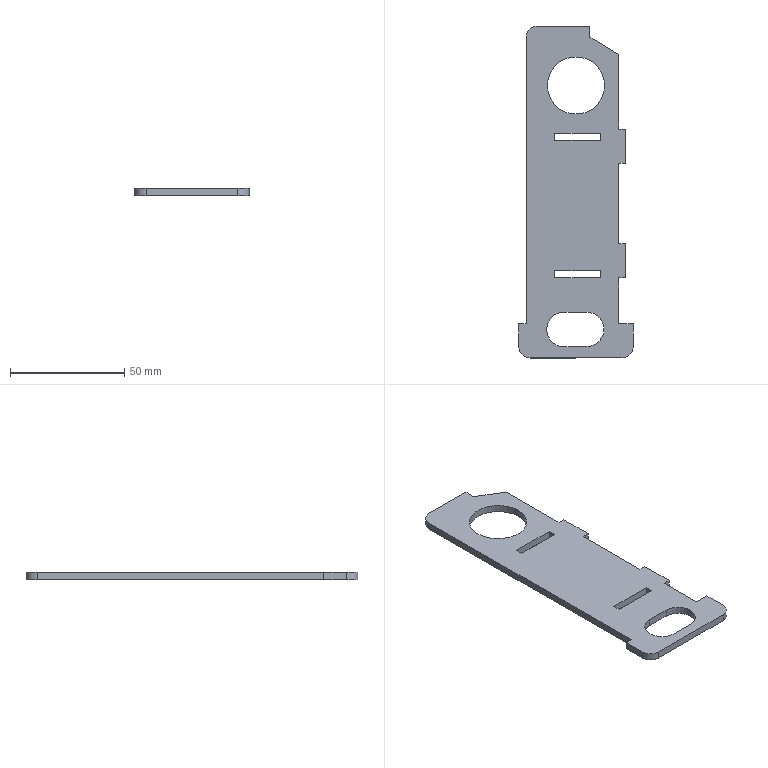Part | SolidWorks | features Fillet 1, FlatPattern 1, SMBaseFlange 1, SheetMetal 1 | 1 solid | 38 faces | box 50 x 145 x 3.2 mm | volume 16071 mm3 | plane 30 | cylinder 8 | commonest cylinder face diameters 10 x3 15 x3 25 x2
STEP:
#1=CARTESIAN_POINT('',(3.442,-44.557,-3.2));
#2=VERTEX_POINT('',#1);
#3=CARTESIAN_POINT('',(-4.058,-37.057,-3.2));
#4=VERTEX_POINT('',#3);
#5=CARTESIAN_POINT('',(-4.058,-44.557,-3.2));
#6=DIRECTION('',(0.,0.,1.));
#7=DIRECTION('',(1.,0.,0.));
#8=AXIS2_PLACEMENT_3D('',#5,#6,#7);
#9=CIRCLE('',#8,7.5);
#10=EDGE_CURVE('',#2,#4,#9,.T.);
#11=ORIENTED_EDGE('',*,*,#10,.F.);
#12=CARTESIAN_POINT('',(3.442,-44.557,0.));
#13=VERTEX_POINT('',#12);
#14=CARTESIAN_POINT('',(3.442,-44.557,-3.2));
#15=DIRECTION('',(0.,0.,1.));
#16=VECTOR('',#15,1000.);
#17=LINE('',#14,#16);
#18=EDGE_CURVE('',#2,#13,#17,.T.);
#19=ORIENTED_EDGE('',*,*,#18,.T.);
#20=CARTESIAN_POINT('',(-4.058,-37.057,0.));
#21=VERTEX_POINT('',#20);
#22=CARTESIAN_POINT('',(-4.058,-44.557,0.));
#23=DIRECTION('',(0.,0.,1.));
#24=DIRECTION('',(1.,0.,0.));
#25=AXIS2_PLACEMENT_3D('',#22,#23,#24);
#26=CIRCLE('',#25,7.5);
#27=EDGE_CURVE('',#13,#21,#26,.T.);
#28=ORIENTED_EDGE('',*,*,#27,.T.);
#29=CARTESIAN_POINT('',(-4.058,-37.057,-3.2));
#30=DIRECTION('',(0.,0.,1.));
#31=VECTOR('',#30,1000.);
#32=LINE('',#29,#31);
#33=EDGE_CURVE('',#4,#21,#32,.T.);
#34=ORIENTED_EDGE('',*,*,#33,.F.);
#35=EDGE_LOOP('',(#11,#19,#28,#34));
#36=FACE_OUTER_BOUND('',#35,.T.);
#37=CARTESIAN_POINT('',(-4.058,-44.557,-3.2));
#38=DIRECTION('',(0.,0.,1.));
#39=DIRECTION('',(1.,0.,0.));
#40=AXIS2_PLACEMENT_3D('',#37,#38,#39);
#41=CYLINDRICAL_SURFACE('',#40,7.5);
#42=ADVANCED_FACE('',(#36),#41,.F.);
#43=CARTESIAN_POINT('',(-21.258,61.943,-3.2));
#44=VERTEX_POINT('',#43);
#45=CARTESIAN_POINT('',(3.742,61.943,-3.2));
#46=VERTEX_POINT('',#45);
#47=CARTESIAN_POINT('',(-8.758,61.943,-3.2));
#48=DIRECTION('',(0.,0.,1.));
#49=DIRECTION('',(1.,0.,0.));
#50=AXIS2_PLACEMENT_3D('',#47,#48,#49);
#51=CIRCLE('',#50,12.5);
#52=EDGE_CURVE('',#44,#46,#51,.T.);
#53=ORIENTED_EDGE('',*,*,#52,.F.);
#54=CARTESIAN_POINT('',(-21.258,61.943,0.));
#55=VERTEX_POINT('',#54);
#56=CARTESIAN_POINT('',(-21.258,61.943,-3.2));
#57=DIRECTION('',(0.,0.,1.));
#58=VECTOR('',#57,1000.);
#59=LINE('',#56,#58);
#60=EDGE_CURVE('',#44,#55,#59,.T.);
#61=ORIENTED_EDGE('',*,*,#60,.T.);
#62=CARTESIAN_POINT('',(3.742,61.943,0.));
#63=VERTEX_POINT('',#62);
#64=CARTESIAN_POINT('',(-8.758,61.943,0.));
#65=DIRECTION('',(0.,0.,1.));
#66=DIRECTION('',(1.,0.,0.));
#67=AXIS2_PLACEMENT_3D('',#64,#65,#66);
#68=CIRCLE('',#67,12.5);
#69=EDGE_CURVE('',#55,#63,#68,.T.);
#70=ORIENTED_EDGE('',*,*,#69,.T.);
#71=CARTESIAN_POINT('',(3.742,61.943,-3.2));
#72=DIRECTION('',(0.,0.,1.));
#73=VECTOR('',#72,1000.);
#74=LINE('',#71,#73);
#75=EDGE_CURVE('',#46,#63,#74,.T.);
#76=ORIENTED_EDGE('',*,*,#75,.F.);
#77=EDGE_LOOP('',(#53,#61,#70,#76));
#78=FACE_OUTER_BOUND('',#77,.T.);
#79=CARTESIAN_POINT('',(-8.758,61.943,-3.2));
#80=DIRECTION('',(0.,0.,1.));
#81=DIRECTION('',(1.,0.,0.));
#82=AXIS2_PLACEMENT_3D('',#79,#80,#81);
#83=CYLINDRICAL_SURFACE('',#82,12.5);
#84=ADVANCED_FACE('',(#78),#83,.F.);
#85=CARTESIAN_POINT('',(-28.758,-57.057,0.));
#86=VERTEX_POINT('',#85);
#87=CARTESIAN_POINT('',(11.242,-57.057,0.));
#88=VERTEX_POINT('',#87);
#89=CARTESIAN_POINT('',(16.242,-57.057,0.));
#90=DIRECTION('',(1.,0.,0.));
#91=VECTOR('',#90,1000.);
#92=LINE('',#89,#91);
#93=EDGE_CURVE('',#86,#88,#92,.T.);
#94=ORIENTED_EDGE('',*,*,#93,.F.);
#95=CARTESIAN_POINT('',(-28.758,-57.057,-3.2));
#96=VERTEX_POINT('',#95);
#97=CARTESIAN_POINT('',(-28.758,-57.057,-3.2));
#98=DIRECTION('',(0.,0.,-1.));
#99=VECTOR('',#98,1000.);
#100=LINE('',#97,#99);
#101=EDGE_CURVE('',#86,#96,#100,.T.);
#102=ORIENTED_EDGE('',*,*,#101,.T.);
#103=CARTESIAN_POINT('',(11.242,-57.057,-3.2));
#104=VERTEX_POINT('',#103);
#105=CARTESIAN_POINT('',(16.242,-57.057,-3.2));
#106=DIRECTION('',(1.,0.,0.));
#107=VECTOR('',#106,1000.);
#108=LINE('',#105,#107);
#109=EDGE_CURVE('',#96,#104,#108,.T.);
#110=ORIENTED_EDGE('',*,*,#109,.T.);
#111=CARTESIAN_POINT('',(11.242,-57.057,-3.2));
#112=DIRECTION('',(0.,0.,1.));
#113=VECTOR('',#112,1000.);
#114=LINE('',#111,#113);
#115=EDGE_CURVE('',#104,#88,#114,.T.);
#116=ORIENTED_EDGE('',*,*,#115,.T.);
#117=EDGE_LOOP('',(#94,#102,#110,#116));
#118=FACE_OUTER_BOUND('',#117,.T.);
#119=CARTESIAN_POINT('',(16.242,-57.057,-3.2));
#120=DIRECTION('',(0.,-1.,0.));
#121=DIRECTION('',(1.,0.,0.));
#122=AXIS2_PLACEMENT_3D('',#119,#120,#121);
#123=PLANE('',#122);
#124=ADVANCED_FACE('',(#118),#123,.T.);
#125=CARTESIAN_POINT('',(-33.758,-42.057,-3.2));
#126=VERTEX_POINT('',#125);
#127=CARTESIAN_POINT('',(-33.758,-52.057,-3.2));
#128=VERTEX_POINT('',#127);
#129=CARTESIAN_POINT('',(-33.758,-57.057,-3.2));
#130=DIRECTION('',(0.,-1.,0.));
#131=VECTOR('',#130,1000.);
#132=LINE('',#129,#131);
#133=EDGE_CURVE('',#126,#128,#132,.T.);
#134=ORIENTED_EDGE('',*,*,#133,.T.);
#135=CARTESIAN_POINT('',(-33.758,-52.057,0.));
#136=VERTEX_POINT('',#135);
#137=CARTESIAN_POINT('',(-33.758,-52.057,-3.2));
#138=DIRECTION('',(0.,0.,1.));
#139=VECTOR('',#138,1000.);
#140=LINE('',#137,#139);
#141=EDGE_CURVE('',#128,#136,#140,.T.);
#142=ORIENTED_EDGE('',*,*,#141,.T.);
#143=CARTESIAN_POINT('',(-33.758,-42.057,0.));
#144=VERTEX_POINT('',#143);
#145=CARTESIAN_POINT('',(-33.758,-57.057,0.));
#146=DIRECTION('',(0.,-1.,0.));
#147=VECTOR('',#146,1000.);
#148=LINE('',#145,#147);
#149=EDGE_CURVE('',#144,#136,#148,.T.);
#150=ORIENTED_EDGE('',*,*,#149,.F.);
#151=CARTESIAN_POINT('',(-33.758,-42.057,-3.2));
#152=DIRECTION('',(0.,0.,1.));
#153=VECTOR('',#152,1000.);
#154=LINE('',#151,#153);
#155=EDGE_CURVE('',#126,#144,#154,.T.);
#156=ORIENTED_EDGE('',*,*,#155,.F.);
#157=EDGE_LOOP('',(#134,#142,#150,#156));
#158=FACE_OUTER_BOUND('',#157,.T.);
#159=CARTESIAN_POINT('',(-33.758,-57.057,-3.2));
#160=DIRECTION('',(-1.,0.,0.));
#161=DIRECTION('',(0.,-1.,0.));
#162=AXIS2_PLACEMENT_3D('',#159,#160,#161);
#163=PLANE('',#162);
#164=ADVANCED_FACE('',(#158),#163,.T.);
#165=CARTESIAN_POINT('',(-30.558,-42.057,0.));
#166=VERTEX_POINT('',#165);
#167=CARTESIAN_POINT('',(-33.758,-42.057,0.));
#168=DIRECTION('',(-1.,0.,0.));
#169=VECTOR('',#168,1000.);
#170=LINE('',#167,#169);
#171=EDGE_CURVE('',#166,#144,#170,.T.);
#172=ORIENTED_EDGE('',*,*,#171,.F.);
#173=CARTESIAN_POINT('',(-30.558,-42.057,-3.2));
#174=VERTEX_POINT('',#173);
#175=CARTESIAN_POINT('',(-30.558,-42.057,-3.2));
#176=DIRECTION('',(0.,0.,1.));
#177=VECTOR('',#176,1000.);
#178=LINE('',#175,#177);
#179=EDGE_CURVE('',#174,#166,#178,.T.);
#180=ORIENTED_EDGE('',*,*,#179,.F.);
#181=CARTESIAN_POINT('',(-33.758,-42.057,-3.2));
#182=DIRECTION('',(-1.,0.,0.));
#183=VECTOR('',#182,1000.);
#184=LINE('',#181,#183);
#185=EDGE_CURVE('',#174,#126,#184,.T.);
#186=ORIENTED_EDGE('',*,*,#185,.T.);
#187=ORIENTED_EDGE('',*,*,#155,.T.);
#188=EDGE_LOOP('',(#172,#180,#186,#187));
#189=FACE_OUTER_BOUND('',#188,.T.);
#190=CARTESIAN_POINT('',(-33.758,-42.057,-3.2));
#191=DIRECTION('',(0.,1.,0.));
#192=DIRECTION('',(-1.,0.,0.));
#193=AXIS2_PLACEMENT_3D('',#190,#191,#192);
#194=PLANE('',#193);
#195=ADVANCED_FACE('',(#189),#194,.T.);
#196=CARTESIAN_POINT('',(-30.558,82.943,0.));
#197=VERTEX_POINT('',#196);
#198=CARTESIAN_POINT('',(-30.558,-42.057,0.));
#199=DIRECTION('',(0.,-1.,0.));
#200=VECTOR('',#199,1000.);
#201=LINE('',#198,#200);
#202=EDGE_CURVE('',#197,#166,#201,.T.);
#203=ORIENTED_EDGE('',*,*,#202,.F.);
#204=CARTESIAN_POINT('',(-30.558,82.943,-3.2));
#205=VERTEX_POINT('',#204);
#206=CARTESIAN_POINT('',(-30.558,82.943,-3.2));
#207=DIRECTION('',(0.,0.,-1.));
#208=VECTOR('',#207,1000.);
#209=LINE('',#206,#208);
#210=EDGE_CURVE('',#197,#205,#209,.T.);
#211=ORIENTED_EDGE('',*,*,#210,.T.);
#212=CARTESIAN_POINT('',(-30.558,-42.057,-3.2));
#213=DIRECTION('',(0.,-1.,0.));
#214=VECTOR('',#213,1000.);
#215=LINE('',#212,#214);
#216=EDGE_CURVE('',#205,#174,#215,.T.);
#217=ORIENTED_EDGE('',*,*,#216,.T.);
#218=ORIENTED_EDGE('',*,*,#179,.T.);
#219=EDGE_LOOP('',(#203,#211,#217,#218));
#220=FACE_OUTER_BOUND('',#219,.T.);
#221=CARTESIAN_POINT('',(-30.558,-42.057,-3.2));
#222=DIRECTION('',(-1.,0.,0.));
#223=DIRECTION('',(0.,0.,1.));
#224=AXIS2_PLACEMENT_3D('',#221,#222,#223);
#225=PLANE('',#224);
#226=ADVANCED_FACE('',(#220),#225,.T.);
#227=CARTESIAN_POINT('',(-2.658,87.943,-3.2));
#228=VERTEX_POINT('',#227);
#229=CARTESIAN_POINT('',(-25.558,87.943,-3.2));
#230=VERTEX_POINT('',#229);
#231=CARTESIAN_POINT('',(-30.558,87.943,-3.2));
#232=DIRECTION('',(-1.,0.,0.));
#233=VECTOR('',#232,1000.);
#234=LINE('',#231,#233);
#235=EDGE_CURVE('',#228,#230,#234,.T.);
#236=ORIENTED_EDGE('',*,*,#235,.T.);
#237=CARTESIAN_POINT('',(-25.558,87.943,0.));
#238=VERTEX_POINT('',#237);
#239=CARTESIAN_POINT('',(-25.558,87.943,-3.2));
#240=DIRECTION('',(0.,0.,1.));
#241=VECTOR('',#240,1000.);
#242=LINE('',#239,#241);
#243=EDGE_CURVE('',#230,#238,#242,.T.);
#244=ORIENTED_EDGE('',*,*,#243,.T.);
#245=CARTESIAN_POINT('',(-2.658,87.943,0.));
#246=VERTEX_POINT('',#245);
#247=CARTESIAN_POINT('',(-30.558,87.943,0.));
#248=DIRECTION('',(-1.,0.,0.));
#249=VECTOR('',#248,1000.);
#250=LINE('',#247,#249);
#251=EDGE_CURVE('',#246,#238,#250,.T.);
#252=ORIENTED_EDGE('',*,*,#251,.F.);
#253=CARTESIAN_POINT('',(-2.658,87.943,-3.2));
#254=DIRECTION('',(0.,0.,1.));
#255=VECTOR('',#254,1000.);
#256=LINE('',#253,#255);
#257=EDGE_CURVE('',#228,#246,#256,.T.);
#258=ORIENTED_EDGE('',*,*,#257,.F.);
#259=EDGE_LOOP('',(#236,#244,#252,#258));
#260=FACE_OUTER_BOUND('',#259,.T.);
#261=CARTESIAN_POINT('',(-30.558,87.943,-3.2));
#262=DIRECTION('',(0.,1.,0.));
#263=DIRECTION('',(0.,0.,1.));
#264=AXIS2_PLACEMENT_3D('',#261,#262,#263);
#265=PLANE('',#264);
#266=ADVANCED_FACE('',(#260),#265,.T.);
#267=CARTESIAN_POINT('',(-2.658,83.075,0.));
#268=VERTEX_POINT('',#267);
#269=CARTESIAN_POINT('',(-2.658,87.943,0.));
#270=DIRECTION('',(0.,1.,0.));
#271=VECTOR('',#270,1000.);
#272=LINE('',#269,#271);
#273=EDGE_CURVE('',#268,#246,#272,.T.);
#274=ORIENTED_EDGE('',*,*,#273,.F.);
#275=CARTESIAN_POINT('',(-2.658,83.075,-3.2));
#276=VERTEX_POINT('',#275);
#277=CARTESIAN_POINT('',(-2.658,83.075,-3.2));
#278=DIRECTION('',(0.,0.,1.));
#279=VECTOR('',#278,1000.);
#280=LINE('',#277,#279);
#281=EDGE_CURVE('',#276,#268,#280,.T.);
#282=ORIENTED_EDGE('',*,*,#281,.F.);
#283=CARTESIAN_POINT('',(-2.658,87.943,-3.2));
#284=DIRECTION('',(0.,1.,0.));
#285=VECTOR('',#284,1000.);
#286=LINE('',#283,#285);
#287=EDGE_CURVE('',#276,#228,#286,.T.);
#288=ORIENTED_EDGE('',*,*,#287,.T.);
#289=ORIENTED_EDGE('',*,*,#257,.T.);
#290=EDGE_LOOP('',(#274,#282,#288,#289));
#291=FACE_OUTER_BOUND('',#290,.T.);
#292=CARTESIAN_POINT('',(-2.658,87.943,-3.2));
#293=DIRECTION('',(1.,0.,0.));
#294=DIRECTION('',(0.,1.,0.));
#295=AXIS2_PLACEMENT_3D('',#292,#293,#294);
#296=PLANE('',#295);
#297=ADVANCED_FACE('',(#291),#296,.T.);
#298=CARTESIAN_POINT('',(9.842,75.486,0.));
#299=VERTEX_POINT('',#298);
#300=CARTESIAN_POINT('',(9.842,75.486,0.));
#301=DIRECTION('',(-0.8548,0.519,0.));
#302=VECTOR('',#301,1000.);
#303=LINE('',#300,#302);
#304=EDGE_CURVE('',#299,#268,#303,.T.);
#305=ORIENTED_EDGE('',*,*,#304,.F.);
#306=CARTESIAN_POINT('',(9.842,75.486,-3.2));
#307=VERTEX_POINT('',#306);
#308=CARTESIAN_POINT('',(9.842,75.486,-3.2));
#309=DIRECTION('',(0.,0.,1.));
#310=VECTOR('',#309,1000.);
#311=LINE('',#308,#310);
#312=EDGE_CURVE('',#307,#299,#311,.T.);
#313=ORIENTED_EDGE('',*,*,#312,.F.);
#314=CARTESIAN_POINT('',(9.842,75.486,-3.2));
#315=DIRECTION('',(-0.8548,0.519,0.));
#316=VECTOR('',#315,1000.);
#317=LINE('',#314,#316);
#318=EDGE_CURVE('',#307,#276,#317,.T.);
#319=ORIENTED_EDGE('',*,*,#318,.T.);
#320=ORIENTED_EDGE('',*,*,#281,.T.);
#321=EDGE_LOOP('',(#305,#313,#319,#320));
#322=FACE_OUTER_BOUND('',#321,.T.);
#323=CARTESIAN_POINT('',(9.842,75.486,-3.2));
#324=DIRECTION('',(0.519,0.8548,0.));
#325=DIRECTION('',(-0.8548,0.519,0.));
#326=AXIS2_PLACEMENT_3D('',#323,#324,#325);
#327=PLANE('',#326);
#328=ADVANCED_FACE('',(#322),#327,.T.);
#329=CARTESIAN_POINT('',(9.842,42.943,0.));
#330=VERTEX_POINT('',#329);
#331=CARTESIAN_POINT('',(9.842,75.486,0.));
#332=DIRECTION('',(0.,1.,0.));
#333=VECTOR('',#332,1000.);
#334=LINE('',#331,#333);
#335=EDGE_CURVE('',#330,#299,#334,.T.);
#336=ORIENTED_EDGE('',*,*,#335,.F.);
#337=CARTESIAN_POINT('',(9.842,42.943,-3.2));
#338=VERTEX_POINT('',#337);
#339=CARTESIAN_POINT('',(9.842,42.943,-3.2));
#340=DIRECTION('',(0.,0.,1.));
#341=VECTOR('',#340,1000.);
#342=LINE('',#339,#341);
#343=EDGE_CURVE('',#338,#330,#342,.T.);
#344=ORIENTED_EDGE('',*,*,#343,.F.);
#345=CARTESIAN_POINT('',(9.842,75.486,-3.2));
#346=DIRECTION('',(0.,1.,0.));
#347=VECTOR('',#346,1000.);
#348=LINE('',#345,#347);
#349=EDGE_CURVE('',#338,#307,#348,.T.);
#350=ORIENTED_EDGE('',*,*,#349,.T.);
#351=ORIENTED_EDGE('',*,*,#312,.T.);
#352=EDGE_LOOP('',(#336,#344,#350,#351));
#353=FACE_OUTER_BOUND('',#352,.T.);
#354=CARTESIAN_POINT('',(9.842,75.486,-3.2));
#355=DIRECTION('',(1.,0.,0.));
#356=DIRECTION('',(0.,0.,-1.));
#357=AXIS2_PLACEMENT_3D('',#354,#355,#356);
#358=PLANE('',#357);
#359=ADVANCED_FACE('',(#353),#358,.T.);
#360=CARTESIAN_POINT('',(12.842,42.943,0.));
#361=VERTEX_POINT('',#360);
#362=CARTESIAN_POINT('',(9.842,42.943,0.));
#363=DIRECTION('',(-1.,0.,0.));
#364=VECTOR('',#363,1000.);
#365=LINE('',#362,#364);
#366=EDGE_CURVE('',#361,#330,#365,.T.);
#367=ORIENTED_EDGE('',*,*,#366,.F.);
#368=CARTESIAN_POINT('',(12.842,42.943,-3.2));
#369=VERTEX_POINT('',#368);
#370=CARTESIAN_POINT('',(12.842,42.943,-3.2));
#371=DIRECTION('',(0.,0.,1.));
#372=VECTOR('',#371,1000.);
#373=LINE('',#370,#372);
#374=EDGE_CURVE('',#369,#361,#373,.T.);
#375=ORIENTED_EDGE('',*,*,#374,.F.);
#376=CARTESIAN_POINT('',(9.842,42.943,-3.2));
#377=DIRECTION('',(-1.,0.,0.));
#378=VECTOR('',#377,1000.);
#379=LINE('',#376,#378);
#380=EDGE_CURVE('',#369,#338,#379,.T.);
#381=ORIENTED_EDGE('',*,*,#380,.T.);
#382=ORIENTED_EDGE('',*,*,#343,.T.);
#383=EDGE_LOOP('',(#367,#375,#381,#382));
#384=FACE_OUTER_BOUND('',#383,.T.);
#385=CARTESIAN_POINT('',(9.842,42.943,-3.2));
#386=DIRECTION('',(0.,1.,0.));
#387=DIRECTION('',(0.,0.,1.));
#388=AXIS2_PLACEMENT_3D('',#385,#386,#387);
#389=PLANE('',#388);
#390=ADVANCED_FACE('',(#384),#389,.T.);
#391=CARTESIAN_POINT('',(12.842,27.943,0.));
#392=VERTEX_POINT('',#391);
#393=CARTESIAN_POINT('',(12.842,42.943,0.));
#394=DIRECTION('',(0.,1.,0.));
#395=VECTOR('',#394,1000.);
#396=LINE('',#393,#395);
#397=EDGE_CURVE('',#392,#361,#396,.T.);
#398=ORIENTED_EDGE('',*,*,#397,.F.);
#399=CARTESIAN_POINT('',(12.842,27.943,-3.2));
#400=VERTEX_POINT('',#399);
#401=CARTESIAN_POINT('',(12.842,27.943,-3.2));
#402=DIRECTION('',(0.,0.,1.));
#403=VECTOR('',#402,1000.);
#404=LINE('',#401,#403);
#405=EDGE_CURVE('',#400,#392,#404,.T.);
#406=ORIENTED_EDGE('',*,*,#405,.F.);
#407=CARTESIAN_POINT('',(12.842,42.943,-3.2));
#408=DIRECTION('',(0.,1.,0.));
#409=VECTOR('',#408,1000.);
#410=LINE('',#407,#409);
#411=EDGE_CURVE('',#400,#369,#410,.T.);
#412=ORIENTED_EDGE('',*,*,#411,.T.);
#413=ORIENTED_EDGE('',*,*,#374,.T.);
#414=EDGE_LOOP('',(#398,#406,#412,#413));
#415=FACE_OUTER_BOUND('',#414,.T.);
#416=CARTESIAN_POINT('',(12.842,42.943,-3.2));
#417=DIRECTION('',(1.,0.,0.));
#418=DIRECTION('',(0.,0.,-1.));
#419=AXIS2_PLACEMENT_3D('',#416,#417,#418);
#420=PLANE('',#419);
#421=ADVANCED_FACE('',(#415),#420,.T.);
#422=CARTESIAN_POINT('',(9.842,27.943,0.));
#423=VERTEX_POINT('',#422);
#424=CARTESIAN_POINT('',(12.842,27.943,0.));
#425=DIRECTION('',(1.,0.,0.));
#426=VECTOR('',#425,1000.);
#427=LINE('',#424,#426);
#428=EDGE_CURVE('',#423,#392,#427,.T.);
#429=ORIENTED_EDGE('',*,*,#428,.F.);
#430=CARTESIAN_POINT('',(9.842,27.943,-3.2));
#431=VERTEX_POINT('',#430);
#432=CARTESIAN_POINT('',(9.842,27.943,-3.2));
#433=DIRECTION('',(0.,0.,1.));
#434=VECTOR('',#433,1000.);
#435=LINE('',#432,#434);
#436=EDGE_CURVE('',#431,#423,#435,.T.);
#437=ORIENTED_EDGE('',*,*,#436,.F.);
#438=CARTESIAN_POINT('',(12.842,27.943,-3.2));
#439=DIRECTION('',(1.,0.,0.));
#440=VECTOR('',#439,1000.);
#441=LINE('',#438,#440);
#442=EDGE_CURVE('',#431,#400,#441,.T.);
#443=ORIENTED_EDGE('',*,*,#442,.T.);
#444=ORIENTED_EDGE('',*,*,#405,.T.);
#445=EDGE_LOOP('',(#429,#437,#443,#444));
#446=FACE_OUTER_BOUND('',#445,.T.);
#447=CARTESIAN_POINT('',(12.842,27.943,-3.2));
#448=DIRECTION('',(0.,-1.,0.));
#449=DIRECTION('',(0.,0.,-1.));
#450=AXIS2_PLACEMENT_3D('',#447,#448,#449);
#451=PLANE('',#450);
#452=ADVANCED_FACE('',(#446),#451,.T.);
#453=CARTESIAN_POINT('',(9.842,-7.057,0.));
#454=VERTEX_POINT('',#453);
#455=CARTESIAN_POINT('',(9.842,27.943,0.));
#456=DIRECTION('',(0.,1.,0.));
#457=VECTOR('',#456,1000.);
#458=LINE('',#455,#457);
#459=EDGE_CURVE('',#454,#423,#458,.T.);
#460=ORIENTED_EDGE('',*,*,#459,.F.);
#461=CARTESIAN_POINT('',(9.842,-7.057,-3.2));
#462=VERTEX_POINT('',#461);
#463=CARTESIAN_POINT('',(9.842,-7.057,-3.2));
#464=DIRECTION('',(0.,0.,1.));
#465=VECTOR('',#464,1000.);
#466=LINE('',#463,#465);
#467=EDGE_CURVE('',#462,#454,#466,.T.);
#468=ORIENTED_EDGE('',*,*,#467,.F.);
#469=CARTESIAN_POINT('',(9.842,27.943,-3.2));
#470=DIRECTION('',(0.,1.,0.));
#471=VECTOR('',#470,1000.);
#472=LINE('',#469,#471);
#473=EDGE_CURVE('',#462,#431,#472,.T.);
#474=ORIENTED_EDGE('',*,*,#473,.T.);
#475=ORIENTED_EDGE('',*,*,#436,.T.);
#476=EDGE_LOOP('',(#460,#468,#474,#475));
#477=FACE_OUTER_BOUND('',#476,.T.);
#478=CARTESIAN_POINT('',(9.842,27.943,-3.2));
#479=DIRECTION('',(1.,0.,0.));
#480=DIRECTION('',(0.,1.,0.));
#481=AXIS2_PLACEMENT_3D('',#478,#479,#480);
#482=PLANE('',#481);
#483=ADVANCED_FACE('',(#477),#482,.T.);
#484=CARTESIAN_POINT('',(12.842,-7.057,0.));
#485=VERTEX_POINT('',#484);
#486=CARTESIAN_POINT('',(9.842,-7.057,0.));
#487=DIRECTION('',(-1.,0.,0.));
#488=VECTOR('',#487,1000.);
#489=LINE('',#486,#488);
#490=EDGE_CURVE('',#485,#454,#489,.T.);
#491=ORIENTED_EDGE('',*,*,#490,.F.);
#492=CARTESIAN_POINT('',(12.842,-7.057,-3.2));
#493=VERTEX_POINT('',#492);
#494=CARTESIAN_POINT('',(12.842,-7.057,-3.2));
#495=DIRECTION('',(0.,0.,1.));
#496=VECTOR('',#495,1000.);
#497=LINE('',#494,#496);
#498=EDGE_CURVE('',#493,#485,#497,.T.);
#499=ORIENTED_EDGE('',*,*,#498,.F.);
#500=CARTESIAN_POINT('',(9.842,-7.057,-3.2));
#501=DIRECTION('',(-1.,0.,0.));
#502=VECTOR('',#501,1000.);
#503=LINE('',#500,#502);
#504=EDGE_CURVE('',#493,#462,#503,.T.);
#505=ORIENTED_EDGE('',*,*,#504,.T.);
#506=ORIENTED_EDGE('',*,*,#467,.T.);
#507=EDGE_LOOP('',(#491,#499,#505,#506));
#508=FACE_OUTER_BOUND('',#507,.T.);
#509=CARTESIAN_POINT('',(9.842,-7.057,-3.2));
#510=DIRECTION('',(0.,1.,0.));
#511=DIRECTION('',(0.,0.,1.));
#512=AXIS2_PLACEMENT_3D('',#509,#510,#511);
#513=PLANE('',#512);
#514=ADVANCED_FACE('',(#508),#513,.T.);
#515=CARTESIAN_POINT('',(12.842,-22.057,0.));
#516=VERTEX_POINT('',#515);
#517=CARTESIAN_POINT('',(12.842,-7.057,0.));
#518=DIRECTION('',(0.,1.,0.));
#519=VECTOR('',#518,1000.);
#520=LINE('',#517,#519);
#521=EDGE_CURVE('',#516,#485,#520,.T.);
#522=ORIENTED_EDGE('',*,*,#521,.F.);
#523=CARTESIAN_POINT('',(12.842,-22.057,-3.2));
#524=VERTEX_POINT('',#523);
#525=CARTESIAN_POINT('',(12.842,-22.057,-3.2));
#526=DIRECTION('',(0.,0.,1.));
#527=VECTOR('',#526,1000.);
#528=LINE('',#525,#527);
#529=EDGE_CURVE('',#524,#516,#528,.T.);
#530=ORIENTED_EDGE('',*,*,#529,.F.);
#531=CARTESIAN_POINT('',(12.842,-7.057,-3.2));
#532=DIRECTION('',(0.,1.,0.));
#533=VECTOR('',#532,1000.);
#534=LINE('',#531,#533);
#535=EDGE_CURVE('',#524,#493,#534,.T.);
#536=ORIENTED_EDGE('',*,*,#535,.T.);
#537=ORIENTED_EDGE('',*,*,#498,.T.);
#538=EDGE_LOOP('',(#522,#530,#536,#537));
#539=FACE_OUTER_BOUND('',#538,.T.);
#540=CARTESIAN_POINT('',(12.842,-7.057,-3.2));
#541=DIRECTION('',(1.,0.,0.));
#542=DIRECTION('',(0.,0.,-1.));
#543=AXIS2_PLACEMENT_3D('',#540,#541,#542);
#544=PLANE('',#543);
#545=ADVANCED_FACE('',(#539),#544,.T.);
#546=CARTESIAN_POINT('',(9.842,-22.057,0.));
#547=VERTEX_POINT('',#546);
#548=CARTESIAN_POINT('',(12.842,-22.057,0.));
#549=DIRECTION('',(1.,0.,0.));
#550=VECTOR('',#549,1000.);
#551=LINE('',#548,#550);
#552=EDGE_CURVE('',#547,#516,#551,.T.);
#553=ORIENTED_EDGE('',*,*,#552,.F.);
#554=CARTESIAN_POINT('',(9.842,-22.057,-3.2));
#555=VERTEX_POINT('',#554);
#556=CARTESIAN_POINT('',(9.842,-22.057,-3.2));
#557=DIRECTION('',(0.,0.,1.));
#558=VECTOR('',#557,1000.);
#559=LINE('',#556,#558);
#560=EDGE_CURVE('',#555,#547,#559,.T.);
#561=ORIENTED_EDGE('',*,*,#560,.F.);
#562=CARTESIAN_POINT('',(12.842,-22.057,-3.2));
#563=DIRECTION('',(1.,0.,0.));
#564=VECTOR('',#563,1000.);
#565=LINE('',#562,#564);
#566=EDGE_CURVE('',#555,#524,#565,.T.);
#567=ORIENTED_EDGE('',*,*,#566,.T.);
#568=ORIENTED_EDGE('',*,*,#529,.T.);
#569=EDGE_LOOP('',(#553,#561,#567,#568));
#570=FACE_OUTER_BOUND('',#569,.T.);
#571=CARTESIAN_POINT('',(12.842,-22.057,-3.2));
#572=DIRECTION('',(0.,-1.,0.));
#573=DIRECTION('',(0.,0.,-1.));
#574=AXIS2_PLACEMENT_3D('',#571,#572,#573);
#575=PLANE('',#574);
#576=ADVANCED_FACE('',(#570),#575,.T.);
#577=CARTESIAN_POINT('',(9.842,-42.057,0.));
#578=VERTEX_POINT('',#577);
#579=CARTESIAN_POINT('',(9.842,-22.057,0.));
#580=DIRECTION('',(0.,1.,0.));
#581=VECTOR('',#580,1000.);
#582=LINE('',#579,#581);
#583=EDGE_CURVE('',#578,#547,#582,.T.);
#584=ORIENTED_EDGE('',*,*,#583,.F.);
#585=CARTESIAN_POINT('',(9.842,-42.057,-3.2));
#586=VERTEX_POINT('',#585);
#587=CARTESIAN_POINT('',(9.842,-42.057,-3.2));
#588=DIRECTION('',(0.,0.,1.));
#589=VECTOR('',#588,1000.);
#590=LINE('',#587,#589);
#591=EDGE_CURVE('',#586,#578,#590,.T.);
#592=ORIENTED_EDGE('',*,*,#591,.F.);
#593=CARTESIAN_POINT('',(9.842,-22.057,-3.2));
#594=DIRECTION('',(0.,1.,0.));
#595=VECTOR('',#594,1000.);
#596=LINE('',#593,#595);
#597=EDGE_CURVE('',#586,#555,#596,.T.);
#598=ORIENTED_EDGE('',*,*,#597,.T.);
#599=ORIENTED_EDGE('',*,*,#560,.T.);
#600=EDGE_LOOP('',(#584,#592,#598,#599));
#601=FACE_OUTER_BOUND('',#600,.T.);
#602=CARTESIAN_POINT('',(9.842,-22.057,-3.2));
#603=DIRECTION('',(1.,0.,0.));
#604=DIRECTION('',(0.,1.,0.));
#605=AXIS2_PLACEMENT_3D('',#602,#603,#604);
#606=PLANE('',#605);
#607=ADVANCED_FACE('',(#601),#606,.T.);
#608=CARTESIAN_POINT('',(16.242,-42.057,0.));
#609=VERTEX_POINT('',#608);
#610=CARTESIAN_POINT('',(16.242,-42.057,0.));
#611=DIRECTION('',(-1.,0.,0.));
#612=VECTOR('',#611,1000.);
#613=LINE('',#610,#612);
#614=EDGE_CURVE('',#609,#578,#613,.T.);
#615=ORIENTED_EDGE('',*,*,#614,.F.);
#616=CARTESIAN_POINT('',(16.242,-42.057,-3.2));
#617=VERTEX_POINT('',#616);
#618=CARTESIAN_POINT('',(16.242,-42.057,-3.2));
#619=DIRECTION('',(0.,0.,1.));
#620=VECTOR('',#619,1000.);
#621=LINE('',#618,#620);
#622=EDGE_CURVE('',#617,#609,#621,.T.);
#623=ORIENTED_EDGE('',*,*,#622,.F.);
#624=CARTESIAN_POINT('',(16.242,-42.057,-3.2));
#625=DIRECTION('',(-1.,0.,0.));
#626=VECTOR('',#625,1000.);
#627=LINE('',#624,#626);
#628=EDGE_CURVE('',#617,#586,#627,.T.);
#629=ORIENTED_EDGE('',*,*,#628,.T.);
#630=ORIENTED_EDGE('',*,*,#591,.T.);
#631=EDGE_LOOP('',(#615,#623,#629,#630));
#632=FACE_OUTER_BOUND('',#631,.T.);
#633=CARTESIAN_POINT('',(16.242,-42.057,-3.2));
#634=DIRECTION('',(0.,1.,0.));
#635=DIRECTION('',(-1.,0.,0.));
#636=AXIS2_PLACEMENT_3D('',#633,#634,#635);
#637=PLANE('',#636);
#638=ADVANCED_FACE('',(#632),#637,.T.);
#639=CARTESIAN_POINT('',(16.242,-52.057,0.));
#640=VERTEX_POINT('',#639);
#641=CARTESIAN_POINT('',(16.242,-42.057,0.));
#642=DIRECTION('',(0.,1.,0.));
#643=VECTOR('',#642,1000.);
#644=LINE('',#641,#643);
#645=EDGE_CURVE('',#640,#609,#644,.T.);
#646=ORIENTED_EDGE('',*,*,#645,.F.);
#647=CARTESIAN_POINT('',(16.242,-52.057,-3.2));
#648=VERTEX_POINT('',#647);
#649=CARTESIAN_POINT('',(16.242,-52.057,-3.2));
#650=DIRECTION('',(0.,0.,-1.));
#651=VECTOR('',#650,1000.);
#652=LINE('',#649,#651);
#653=EDGE_CURVE('',#640,#648,#652,.T.);
#654=ORIENTED_EDGE('',*,*,#653,.T.);
#655=CARTESIAN_POINT('',(16.242,-42.057,-3.2));
#656=DIRECTION('',(0.,1.,0.));
#657=VECTOR('',#656,1000.);
#658=LINE('',#655,#657);
#659=EDGE_CURVE('',#648,#617,#658,.T.);
#660=ORIENTED_EDGE('',*,*,#659,.T.);
#661=ORIENTED_EDGE('',*,*,#622,.T.);
#662=EDGE_LOOP('',(#646,#654,#660,#661));
#663=FACE_OUTER_BOUND('',#662,.T.);
#664=CARTESIAN_POINT('',(16.242,-42.057,-3.2));
#665=DIRECTION('',(1.,0.,0.));
#666=DIRECTION('',(0.,1.,0.));
#667=AXIS2_PLACEMENT_3D('',#664,#665,#666);
#668=PLANE('',#667);
#669=ADVANCED_FACE('',(#663),#668,.T.);
#670=CARTESIAN_POINT('',(-18.058,41.143,-3.2));
#671=VERTEX_POINT('',#670);
#672=CARTESIAN_POINT('',(-18.058,37.943,-3.2));
#673=VERTEX_POINT('',#672);
#674=CARTESIAN_POINT('',(-18.058,37.943,-3.2));
#675=DIRECTION('',(0.,-1.,0.));
#676=VECTOR('',#675,1000.);
#677=LINE('',#674,#676);
#678=EDGE_CURVE('',#671,#673,#677,.T.);
#679=ORIENTED_EDGE('',*,*,#678,.T.);
#680=CARTESIAN_POINT('',(1.942,37.943,-3.2));
#681=VERTEX_POINT('',#680);
#682=CARTESIAN_POINT('',(-18.058,37.943,-3.2));
#683=DIRECTION('',(1.,0.,0.));
#684=VECTOR('',#683,1000.);
#685=LINE('',#682,#684);
#686=EDGE_CURVE('',#673,#681,#685,.T.);
#687=ORIENTED_EDGE('',*,*,#686,.T.);
#688=CARTESIAN_POINT('',(1.942,41.143,-3.2));
#689=VERTEX_POINT('',#688);
#690=CARTESIAN_POINT('',(1.942,37.943,-3.2));
#691=DIRECTION('',(0.,1.,0.));
#692=VECTOR('',#691,1000.);
#693=LINE('',#690,#692);
#694=EDGE_CURVE('',#681,#689,#693,.T.);
#695=ORIENTED_EDGE('',*,*,#694,.T.);
#696=CARTESIAN_POINT('',(-18.058,41.143,-3.2));
#697=DIRECTION('',(-1.,0.,0.));
#698=VECTOR('',#697,1000.);
#699=LINE('',#696,#698);
#700=EDGE_CURVE('',#689,#671,#699,.T.);
#701=ORIENTED_EDGE('',*,*,#700,.T.);
#702=EDGE_LOOP('',(#679,#687,#695,#701));
#703=FACE_BOUND('',#702,.T.);
#704=CARTESIAN_POINT('',(1.942,-22.057,-3.2));
#705=VERTEX_POINT('',#704);
#706=CARTESIAN_POINT('',(1.942,-18.857,-3.2));
#707=VERTEX_POINT('',#706);
#708=CARTESIAN_POINT('',(1.942,-18.857,-3.2));
#709=DIRECTION('',(0.,1.,0.));
#710=VECTOR('',#709,1000.);
#711=LINE('',#708,#710);
#712=EDGE_CURVE('',#705,#707,#711,.T.);
#713=ORIENTED_EDGE('',*,*,#712,.T.);
#714=CARTESIAN_POINT('',(-18.058,-18.857,-3.2));
#715=VERTEX_POINT('',#714);
#716=CARTESIAN_POINT('',(1.942,-18.857,-3.2));
#717=DIRECTION('',(-1.,0.,0.));
#718=VECTOR('',#717,1000.);
#719=LINE('',#716,#718);
#720=EDGE_CURVE('',#707,#715,#719,.T.);
#721=ORIENTED_EDGE('',*,*,#720,.T.);
#722=CARTESIAN_POINT('',(-18.058,-22.057,-3.2));
#723=VERTEX_POINT('',#722);
#724=CARTESIAN_POINT('',(-18.058,-18.857,-3.2));
#725=DIRECTION('',(0.,-1.,0.));
#726=VECTOR('',#725,1000.);
#727=LINE('',#724,#726);
#728=EDGE_CURVE('',#715,#723,#727,.T.);
#729=ORIENTED_EDGE('',*,*,#728,.T.);
#730=CARTESIAN_POINT('',(1.942,-22.057,-3.2));
#731=DIRECTION('',(1.,0.,0.));
#732=VECTOR('',#731,1000.);
#733=LINE('',#730,#732);
#734=EDGE_CURVE('',#723,#705,#733,.T.);
#735=ORIENTED_EDGE('',*,*,#734,.T.);
#736=EDGE_LOOP('',(#713,#721,#729,#735));
#737=FACE_BOUND('',#736,.T.);
#738=CARTESIAN_POINT('',(-4.058,-52.057,-3.2));
#739=VERTEX_POINT('',#738);
#740=CARTESIAN_POINT('',(-4.058,-44.557,-3.2));
#741=DIRECTION('',(0.,0.,1.));
#742=DIRECTION('',(1.,0.,0.));
#743=AXIS2_PLACEMENT_3D('',#740,#741,#742);
#744=CIRCLE('',#743,7.5);
#745=EDGE_CURVE('',#739,#2,#744,.T.);
#746=ORIENTED_EDGE('',*,*,#745,.T.);
#747=ORIENTED_EDGE('',*,*,#10,.T.);
#748=CARTESIAN_POINT('',(-14.058,-37.057,-3.2));
#749=VERTEX_POINT('',#748);
#750=CARTESIAN_POINT('',(-4.058,-37.057,-3.2));
#751=DIRECTION('',(-1.,0.,0.));
#752=VECTOR('',#751,1000.);
#753=LINE('',#750,#752);
#754=EDGE_CURVE('',#4,#749,#753,.T.);
#755=ORIENTED_EDGE('',*,*,#754,.T.);
#756=CARTESIAN_POINT('',(-14.058,-52.057,-3.2));
#757=VERTEX_POINT('',#756);
#758=CARTESIAN_POINT('',(-14.058,-44.557,-3.2));
#759=DIRECTION('',(0.,0.,1.));
#760=DIRECTION('',(1.,0.,0.));
#761=AXIS2_PLACEMENT_3D('',#758,#759,#760);
#762=CIRCLE('',#761,7.5);
#763=EDGE_CURVE('',#749,#757,#762,.T.);
#764=ORIENTED_EDGE('',*,*,#763,.T.);
#765=CARTESIAN_POINT('',(-4.058,-52.057,-3.2));
#766=DIRECTION('',(1.,0.,0.));
#767=VECTOR('',#766,1000.);
#768=LINE('',#765,#767);
#769=EDGE_CURVE('',#757,#739,#768,.T.);
#770=ORIENTED_EDGE('',*,*,#769,.T.);
#771=EDGE_LOOP('',(#746,#747,#755,#764,#770));
#772=FACE_BOUND('',#771,.T.);
#773=CARTESIAN_POINT('',(-8.758,61.943,-3.2));
#774=DIRECTION('',(0.,0.,1.));
#775=DIRECTION('',(1.,0.,0.));
#776=AXIS2_PLACEMENT_3D('',#773,#774,#775);
#777=CIRCLE('',#776,12.5);
#778=EDGE_CURVE('',#46,#44,#777,.T.);
#779=ORIENTED_EDGE('',*,*,#778,.T.);
#780=ORIENTED_EDGE('',*,*,#52,.T.);
#781=EDGE_LOOP('',(#779,#780));
#782=FACE_BOUND('',#781,.T.);
#783=ORIENTED_EDGE('',*,*,#109,.F.);
#784=CARTESIAN_POINT('',(-28.758,-52.057,-3.2));
#785=DIRECTION('',(0.,0.,-1.));
#786=DIRECTION('',(-1.,0.,0.));
#787=AXIS2_PLACEMENT_3D('',#784,#785,#786);
#788=CIRCLE('',#787,5.);
#789=EDGE_CURVE('',#96,#128,#788,.T.);
#790=ORIENTED_EDGE('',*,*,#789,.T.);
#791=ORIENTED_EDGE('',*,*,#133,.F.);
#792=ORIENTED_EDGE('',*,*,#185,.F.);
#793=ORIENTED_EDGE('',*,*,#216,.F.);
#794=CARTESIAN_POINT('',(-25.558,82.943,-3.2));
#795=DIRECTION('',(0.,0.,-1.));
#796=DIRECTION('',(-1.,0.,0.));
#797=AXIS2_PLACEMENT_3D('',#794,#795,#796);
#798=CIRCLE('',#797,5.);
#799=EDGE_CURVE('',#205,#230,#798,.T.);
#800=ORIENTED_EDGE('',*,*,#799,.T.);
#801=ORIENTED_EDGE('',*,*,#235,.F.);
#802=ORIENTED_EDGE('',*,*,#287,.F.);
#803=ORIENTED_EDGE('',*,*,#318,.F.);
#804=ORIENTED_EDGE('',*,*,#349,.F.);
#805=ORIENTED_EDGE('',*,*,#380,.F.);
#806=ORIENTED_EDGE('',*,*,#411,.F.);
#807=ORIENTED_EDGE('',*,*,#442,.F.);
#808=ORIENTED_EDGE('',*,*,#473,.F.);
#809=ORIENTED_EDGE('',*,*,#504,.F.);
#810=ORIENTED_EDGE('',*,*,#535,.F.);
#811=ORIENTED_EDGE('',*,*,#566,.F.);
#812=ORIENTED_EDGE('',*,*,#597,.F.);
#813=ORIENTED_EDGE('',*,*,#628,.F.);
#814=ORIENTED_EDGE('',*,*,#659,.F.);
#815=CARTESIAN_POINT('',(11.242,-52.057,-3.2));
#816=DIRECTION('',(0.,0.,-1.));
#817=DIRECTION('',(-1.,0.,0.));
#818=AXIS2_PLACEMENT_3D('',#815,#816,#817);
#819=CIRCLE('',#818,5.);
#820=EDGE_CURVE('',#648,#104,#819,.T.);
#821=ORIENTED_EDGE('',*,*,#820,.T.);
#822=EDGE_LOOP('',(#783,#790,#791,#792,#793,#800,#801,#802,#803,#804,#805,#806,#807,#808,#809,#810,#811,#812,#813,#814,#821));
#823=FACE_OUTER_BOUND('',#822,.T.);
#824=CARTESIAN_POINT('',(0.,0.,-3.2));
#825=DIRECTION('',(0.,0.,-1.));
#826=DIRECTION('',(-1.,0.,0.));
#827=AXIS2_PLACEMENT_3D('',#824,#825,#826);
#828=PLANE('',#827);
#829=ADVANCED_FACE('',(#703,#737,#772,#782,#823),#828,.T.);
#830=CARTESIAN_POINT('',(-18.058,37.943,0.));
#831=VERTEX_POINT('',#830);
#832=CARTESIAN_POINT('',(1.942,37.943,0.));
#833=VERTEX_POINT('',#832);
#834=CARTESIAN_POINT('',(-18.058,37.943,0.));
#835=DIRECTION('',(1.,0.,0.));
#836=VECTOR('',#835,1000.);
#837=LINE('',#834,#836);
#838=EDGE_CURVE('',#831,#833,#837,.T.);
#839=ORIENTED_EDGE('',*,*,#838,.F.);
#840=CARTESIAN_POINT('',(-18.058,41.143,0.));
#841=VERTEX_POINT('',#840);
#842=CARTESIAN_POINT('',(-18.058,37.943,0.));
#843=DIRECTION('',(0.,-1.,0.));
#844=VECTOR('',#843,1000.);
#845=LINE('',#842,#844);
#846=EDGE_CURVE('',#841,#831,#845,.T.);
#847=ORIENTED_EDGE('',*,*,#846,.F.);
#848=CARTESIAN_POINT('',(1.942,41.143,0.));
#849=VERTEX_POINT('',#848);
#850=CARTESIAN_POINT('',(-18.058,41.143,0.));
#851=DIRECTION('',(-1.,0.,0.));
#852=VECTOR('',#851,1000.);
#853=LINE('',#850,#852);
#854=EDGE_CURVE('',#849,#841,#853,.T.);
#855=ORIENTED_EDGE('',*,*,#854,.F.);
#856=CARTESIAN_POINT('',(1.942,37.943,0.));
#857=DIRECTION('',(0.,1.,0.));
#858=VECTOR('',#857,1000.);
#859=LINE('',#856,#858);
#860=EDGE_CURVE('',#833,#849,#859,.T.);
#861=ORIENTED_EDGE('',*,*,#860,.F.);
#862=EDGE_LOOP('',(#839,#847,#855,#861));
#863=FACE_BOUND('',#862,.T.);
#864=CARTESIAN_POINT('',(1.942,-18.857,0.));
#865=VERTEX_POINT('',#864);
#866=CARTESIAN_POINT('',(-18.058,-18.857,0.));
#867=VERTEX_POINT('',#866);
#868=CARTESIAN_POINT('',(1.942,-18.857,0.));
#869=DIRECTION('',(-1.,0.,0.));
#870=VECTOR('',#869,1000.);
#871=LINE('',#868,#870);
#872=EDGE_CURVE('',#865,#867,#871,.T.);
#873=ORIENTED_EDGE('',*,*,#872,.F.);
#874=CARTESIAN_POINT('',(1.942,-22.057,0.));
#875=VERTEX_POINT('',#874);
#876=CARTESIAN_POINT('',(1.942,-18.857,0.));
#877=DIRECTION('',(0.,1.,0.));
#878=VECTOR('',#877,1000.);
#879=LINE('',#876,#878);
#880=EDGE_CURVE('',#875,#865,#879,.T.);
#881=ORIENTED_EDGE('',*,*,#880,.F.);
#882=CARTESIAN_POINT('',(-18.058,-22.057,0.));
#883=VERTEX_POINT('',#882);
#884=CARTESIAN_POINT('',(1.942,-22.057,0.));
#885=DIRECTION('',(1.,0.,0.));
#886=VECTOR('',#885,1000.);
#887=LINE('',#884,#886);
#888=EDGE_CURVE('',#883,#875,#887,.T.);
#889=ORIENTED_EDGE('',*,*,#888,.F.);
#890=CARTESIAN_POINT('',(-18.058,-18.857,0.));
#891=DIRECTION('',(0.,-1.,0.));
#892=VECTOR('',#891,1000.);
#893=LINE('',#890,#892);
#894=EDGE_CURVE('',#867,#883,#893,.T.);
#895=ORIENTED_EDGE('',*,*,#894,.F.);
#896=EDGE_LOOP('',(#873,#881,#889,#895));
#897=FACE_BOUND('',#896,.T.);
#898=CARTESIAN_POINT('',(-14.058,-37.057,0.));
#899=VERTEX_POINT('',#898);
#900=CARTESIAN_POINT('',(-4.058,-37.057,0.));
#901=DIRECTION('',(-1.,0.,0.));
#902=VECTOR('',#901,1000.);
#903=LINE('',#900,#902);
#904=EDGE_CURVE('',#21,#899,#903,.T.);
#905=ORIENTED_EDGE('',*,*,#904,.F.);
#906=ORIENTED_EDGE('',*,*,#27,.F.);
#907=CARTESIAN_POINT('',(-4.058,-52.057,0.));
#908=VERTEX_POINT('',#907);
#909=CARTESIAN_POINT('',(-4.058,-44.557,0.));
#910=DIRECTION('',(0.,0.,1.));
#911=DIRECTION('',(1.,0.,0.));
#912=AXIS2_PLACEMENT_3D('',#909,#910,#911);
#913=CIRCLE('',#912,7.5);
#914=EDGE_CURVE('',#908,#13,#913,.T.);
#915=ORIENTED_EDGE('',*,*,#914,.F.);
#916=CARTESIAN_POINT('',(-14.058,-52.057,0.));
#917=VERTEX_POINT('',#916);
#918=CARTESIAN_POINT('',(-4.058,-52.057,0.));
#919=DIRECTION('',(1.,0.,0.));
#920=VECTOR('',#919,1000.);
#921=LINE('',#918,#920);
#922=EDGE_CURVE('',#917,#908,#921,.T.);
#923=ORIENTED_EDGE('',*,*,#922,.F.);
#924=CARTESIAN_POINT('',(-14.058,-44.557,0.));
#925=DIRECTION('',(0.,0.,1.));
#926=DIRECTION('',(1.,0.,0.));
#927=AXIS2_PLACEMENT_3D('',#924,#925,#926);
#928=CIRCLE('',#927,7.5);
#929=EDGE_CURVE('',#899,#917,#928,.T.);
#930=ORIENTED_EDGE('',*,*,#929,.F.);
#931=EDGE_LOOP('',(#905,#906,#915,#923,#930));
#932=FACE_BOUND('',#931,.T.);
#933=CARTESIAN_POINT('',(-8.758,61.943,0.));
#934=DIRECTION('',(0.,0.,1.));
#935=DIRECTION('',(1.,0.,0.));
#936=AXIS2_PLACEMENT_3D('',#933,#934,#935);
#937=CIRCLE('',#936,12.5);
#938=EDGE_CURVE('',#63,#55,#937,.T.);
#939=ORIENTED_EDGE('',*,*,#938,.F.);
#940=ORIENTED_EDGE('',*,*,#69,.F.);
#941=EDGE_LOOP('',(#939,#940));
#942=FACE_BOUND('',#941,.T.);
#943=ORIENTED_EDGE('',*,*,#149,.T.);
#944=CARTESIAN_POINT('',(-28.758,-52.057,0.));
#945=DIRECTION('',(0.,0.,1.));
#946=DIRECTION('',(-1.,0.,0.));
#947=AXIS2_PLACEMENT_3D('',#944,#945,#946);
#948=CIRCLE('',#947,5.);
#949=EDGE_CURVE('',#136,#86,#948,.T.);
#950=ORIENTED_EDGE('',*,*,#949,.T.);
#951=ORIENTED_EDGE('',*,*,#93,.T.);
#952=CARTESIAN_POINT('',(11.242,-52.057,0.));
#953=DIRECTION('',(0.,0.,1.));
#954=DIRECTION('',(-1.,0.,0.));
#955=AXIS2_PLACEMENT_3D('',#952,#953,#954);
#956=CIRCLE('',#955,5.);
#957=EDGE_CURVE('',#88,#640,#956,.T.);
#958=ORIENTED_EDGE('',*,*,#957,.T.);
#959=ORIENTED_EDGE('',*,*,#645,.T.);
#960=ORIENTED_EDGE('',*,*,#614,.T.);
#961=ORIENTED_EDGE('',*,*,#583,.T.);
#962=ORIENTED_EDGE('',*,*,#552,.T.);
#963=ORIENTED_EDGE('',*,*,#521,.T.);
#964=ORIENTED_EDGE('',*,*,#490,.T.);
#965=ORIENTED_EDGE('',*,*,#459,.T.);
#966=ORIENTED_EDGE('',*,*,#428,.T.);
#967=ORIENTED_EDGE('',*,*,#397,.T.);
#968=ORIENTED_EDGE('',*,*,#366,.T.);
#969=ORIENTED_EDGE('',*,*,#335,.T.);
#970=ORIENTED_EDGE('',*,*,#304,.T.);
#971=ORIENTED_EDGE('',*,*,#273,.T.);
#972=ORIENTED_EDGE('',*,*,#251,.T.);
#973=CARTESIAN_POINT('',(-25.558,82.943,0.));
#974=DIRECTION('',(0.,0.,1.));
#975=DIRECTION('',(-1.,0.,0.));
#976=AXIS2_PLACEMENT_3D('',#973,#974,#975);
#977=CIRCLE('',#976,5.);
#978=EDGE_CURVE('',#238,#197,#977,.T.);
#979=ORIENTED_EDGE('',*,*,#978,.T.);
#980=ORIENTED_EDGE('',*,*,#202,.T.);
#981=ORIENTED_EDGE('',*,*,#171,.T.);
#982=EDGE_LOOP('',(#943,#950,#951,#958,#959,#960,#961,#962,#963,#964,#965,#966,#967,#968,#969,#970,#971,#972,#979,#980,#981));
#983=FACE_OUTER_BOUND('',#982,.T.);
#984=CARTESIAN_POINT('',(0.,0.,0.));
#985=DIRECTION('',(0.,0.,-1.));
#986=DIRECTION('',(-1.,0.,0.));
#987=AXIS2_PLACEMENT_3D('',#984,#985,#986);
#988=PLANE('',#987);
#989=ADVANCED_FACE('',(#863,#897,#932,#942,#983),#988,.F.);
#990=ORIENTED_EDGE('',*,*,#60,.F.);
#991=ORIENTED_EDGE('',*,*,#778,.F.);
#992=ORIENTED_EDGE('',*,*,#75,.T.);
#993=ORIENTED_EDGE('',*,*,#938,.T.);
#994=EDGE_LOOP('',(#990,#991,#992,#993));
#995=FACE_OUTER_BOUND('',#994,.T.);
#996=CARTESIAN_POINT('',(-8.758,61.943,-3.2));
#997=DIRECTION('',(0.,0.,1.));
#998=DIRECTION('',(1.,0.,0.));
#999=AXIS2_PLACEMENT_3D('',#996,#997,#998);
#1000=CYLINDRICAL_SURFACE('',#999,12.5);
#1001=ADVANCED_FACE('',(#995),#1000,.F.);
#1002=ORIENTED_EDGE('',*,*,#18,.F.);
#1003=ORIENTED_EDGE('',*,*,#745,.F.);
#1004=CARTESIAN_POINT('',(-4.058,-52.057,-3.2));
#1005=DIRECTION('',(0.,0.,1.));
#1006=VECTOR('',#1005,1000.);
#1007=LINE('',#1004,#1006);
#1008=EDGE_CURVE('',#739,#908,#1007,.T.);
#1009=ORIENTED_EDGE('',*,*,#1008,.T.);
#1010=ORIENTED_EDGE('',*,*,#914,.T.);
#1011=EDGE_LOOP('',(#1002,#1003,#1009,#1010));
#1012=FACE_OUTER_BOUND('',#1011,.T.);
#1013=CARTESIAN_POINT('',(-4.058,-44.557,-3.2));
#1014=DIRECTION('',(0.,0.,1.));
#1015=DIRECTION('',(1.,0.,0.));
#1016=AXIS2_PLACEMENT_3D('',#1013,#1014,#1015);
#1017=CYLINDRICAL_SURFACE('',#1016,7.5);
#1018=ADVANCED_FACE('',(#1012),#1017,.F.);
#1019=ORIENTED_EDGE('',*,*,#922,.T.);
#1020=ORIENTED_EDGE('',*,*,#1008,.F.);
#1021=ORIENTED_EDGE('',*,*,#769,.F.);
#1022=CARTESIAN_POINT('',(-14.058,-52.057,-3.2));
#1023=DIRECTION('',(0.,0.,1.));
#1024=VECTOR('',#1023,1000.);
#1025=LINE('',#1022,#1024);
#1026=EDGE_CURVE('',#757,#917,#1025,.T.);
#1027=ORIENTED_EDGE('',*,*,#1026,.T.);
#1028=EDGE_LOOP('',(#1019,#1020,#1021,#1027));
#1029=FACE_OUTER_BOUND('',#1028,.T.);
#1030=CARTESIAN_POINT('',(-4.058,-52.057,-3.2));
#1031=DIRECTION('',(0.,-1.,0.));
#1032=DIRECTION('',(0.,0.,-1.));
#1033=AXIS2_PLACEMENT_3D('',#1030,#1031,#1032);
#1034=PLANE('',#1033);
#1035=ADVANCED_FACE('',(#1029),#1034,.F.);
#1036=ORIENTED_EDGE('',*,*,#929,.T.);
#1037=ORIENTED_EDGE('',*,*,#1026,.F.);
#1038=ORIENTED_EDGE('',*,*,#763,.F.);
#1039=CARTESIAN_POINT('',(-14.058,-37.057,-3.2));
#1040=DIRECTION('',(0.,0.,1.));
#1041=VECTOR('',#1040,1000.);
#1042=LINE('',#1039,#1041);
#1043=EDGE_CURVE('',#749,#899,#1042,.T.);
#1044=ORIENTED_EDGE('',*,*,#1043,.T.);
#1045=EDGE_LOOP('',(#1036,#1037,#1038,#1044));
#1046=FACE_OUTER_BOUND('',#1045,.T.);
#1047=CARTESIAN_POINT('',(-14.058,-44.557,-3.2));
#1048=DIRECTION('',(0.,0.,1.));
#1049=DIRECTION('',(1.,0.,0.));
#1050=AXIS2_PLACEMENT_3D('',#1047,#1048,#1049);
#1051=CYLINDRICAL_SURFACE('',#1050,7.5);
#1052=ADVANCED_FACE('',(#1046),#1051,.F.);
#1053=ORIENTED_EDGE('',*,*,#904,.T.);
#1054=ORIENTED_EDGE('',*,*,#1043,.F.);
#1055=ORIENTED_EDGE('',*,*,#754,.F.);
#1056=ORIENTED_EDGE('',*,*,#33,.T.);
#1057=EDGE_LOOP('',(#1053,#1054,#1055,#1056));
#1058=FACE_OUTER_BOUND('',#1057,.T.);
#1059=CARTESIAN_POINT('',(-4.058,-37.057,-3.2));
#1060=DIRECTION('',(0.,1.,0.));
#1061=DIRECTION('',(0.,0.,1.));
#1062=AXIS2_PLACEMENT_3D('',#1059,#1060,#1061);
#1063=PLANE('',#1062);
#1064=ADVANCED_FACE('',(#1058),#1063,.F.);
#1065=ORIENTED_EDGE('',*,*,#880,.T.);
#1066=CARTESIAN_POINT('',(1.942,-18.857,-3.2));
#1067=DIRECTION('',(0.,0.,1.));
#1068=VECTOR('',#1067,1000.);
#1069=LINE('',#1066,#1068);
#1070=EDGE_CURVE('',#707,#865,#1069,.T.);
#1071=ORIENTED_EDGE('',*,*,#1070,.F.);
#1072=ORIENTED_EDGE('',*,*,#712,.F.);
#1073=CARTESIAN_POINT('',(1.942,-22.057,-3.2));
#1074=DIRECTION('',(0.,0.,1.));
#1075=VECTOR('',#1074,1000.);
#1076=LINE('',#1073,#1075);
#1077=EDGE_CURVE('',#705,#875,#1076,.T.);
#1078=ORIENTED_EDGE('',*,*,#1077,.T.);
#1079=EDGE_LOOP('',(#1065,#1071,#1072,#1078));
#1080=FACE_OUTER_BOUND('',#1079,.T.);
#1081=CARTESIAN_POINT('',(1.942,-18.857,-3.2));
#1082=DIRECTION('',(1.,0.,0.));
#1083=DIRECTION('',(0.,0.,-1.));
#1084=AXIS2_PLACEMENT_3D('',#1081,#1082,#1083);
#1085=PLANE('',#1084);
#1086=ADVANCED_FACE('',(#1080),#1085,.F.);
#1087=ORIENTED_EDGE('',*,*,#888,.T.);
#1088=ORIENTED_EDGE('',*,*,#1077,.F.);
#1089=ORIENTED_EDGE('',*,*,#734,.F.);
#1090=CARTESIAN_POINT('',(-18.058,-22.057,-3.2));
#1091=DIRECTION('',(0.,0.,1.));
#1092=VECTOR('',#1091,1000.);
#1093=LINE('',#1090,#1092);
#1094=EDGE_CURVE('',#723,#883,#1093,.T.);
#1095=ORIENTED_EDGE('',*,*,#1094,.T.);
#1096=EDGE_LOOP('',(#1087,#1088,#1089,#1095));
#1097=FACE_OUTER_BOUND('',#1096,.T.);
#1098=CARTESIAN_POINT('',(1.942,-22.057,-3.2));
#1099=DIRECTION('',(0.,-1.,0.));
#1100=DIRECTION('',(0.,0.,-1.));
#1101=AXIS2_PLACEMENT_3D('',#1098,#1099,#1100);
#1102=PLANE('',#1101);
#1103=ADVANCED_FACE('',(#1097),#1102,.F.);
#1104=ORIENTED_EDGE('',*,*,#894,.T.);
#1105=ORIENTED_EDGE('',*,*,#1094,.F.);
#1106=ORIENTED_EDGE('',*,*,#728,.F.);
#1107=CARTESIAN_POINT('',(-18.058,-18.857,-3.2));
#1108=DIRECTION('',(0.,0.,1.));
#1109=VECTOR('',#1108,1000.);
#1110=LINE('',#1107,#1109);
#1111=EDGE_CURVE('',#715,#867,#1110,.T.);
#1112=ORIENTED_EDGE('',*,*,#1111,.T.);
#1113=EDGE_LOOP('',(#1104,#1105,#1106,#1112));
#1114=FACE_OUTER_BOUND('',#1113,.T.);
#1115=CARTESIAN_POINT('',(-18.058,-18.857,-3.2));
#1116=DIRECTION('',(-1.,0.,0.));
#1117=DIRECTION('',(0.,0.,1.));
#1118=AXIS2_PLACEMENT_3D('',#1115,#1116,#1117);
#1119=PLANE('',#1118);
#1120=ADVANCED_FACE('',(#1114),#1119,.F.);
#1121=ORIENTED_EDGE('',*,*,#872,.T.);
#1122=ORIENTED_EDGE('',*,*,#1111,.F.);
#1123=ORIENTED_EDGE('',*,*,#720,.F.);
#1124=ORIENTED_EDGE('',*,*,#1070,.T.);
#1125=EDGE_LOOP('',(#1121,#1122,#1123,#1124));
#1126=FACE_OUTER_BOUND('',#1125,.T.);
#1127=CARTESIAN_POINT('',(1.942,-18.857,-3.2));
#1128=DIRECTION('',(0.,1.,0.));
#1129=DIRECTION('',(0.,0.,1.));
#1130=AXIS2_PLACEMENT_3D('',#1127,#1128,#1129);
#1131=PLANE('',#1130);
#1132=ADVANCED_FACE('',(#1126),#1131,.F.);
#1133=ORIENTED_EDGE('',*,*,#846,.T.);
#1134=CARTESIAN_POINT('',(-18.058,37.943,-3.2));
#1135=DIRECTION('',(0.,0.,1.));
#1136=VECTOR('',#1135,1000.);
#1137=LINE('',#1134,#1136);
#1138=EDGE_CURVE('',#673,#831,#1137,.T.);
#1139=ORIENTED_EDGE('',*,*,#1138,.F.);
#1140=ORIENTED_EDGE('',*,*,#678,.F.);
#1141=CARTESIAN_POINT('',(-18.058,41.143,-3.2));
#1142=DIRECTION('',(0.,0.,1.));
#1143=VECTOR('',#1142,1000.);
#1144=LINE('',#1141,#1143);
#1145=EDGE_CURVE('',#671,#841,#1144,.T.);
#1146=ORIENTED_EDGE('',*,*,#1145,.T.);
#1147=EDGE_LOOP('',(#1133,#1139,#1140,#1146));
#1148=FACE_OUTER_BOUND('',#1147,.T.);
#1149=CARTESIAN_POINT('',(-18.058,37.943,-3.2));
#1150=DIRECTION('',(-1.,0.,0.));
#1151=DIRECTION('',(0.,0.,1.));
#1152=AXIS2_PLACEMENT_3D('',#1149,#1150,#1151);
#1153=PLANE('',#1152);
#1154=ADVANCED_FACE('',(#1148),#1153,.F.);
#1155=ORIENTED_EDGE('',*,*,#854,.T.);
#1156=ORIENTED_EDGE('',*,*,#1145,.F.);
#1157=ORIENTED_EDGE('',*,*,#700,.F.);
#1158=CARTESIAN_POINT('',(1.942,41.143,-3.2));
#1159=DIRECTION('',(0.,0.,1.));
#1160=VECTOR('',#1159,1000.);
#1161=LINE('',#1158,#1160);
#1162=EDGE_CURVE('',#689,#849,#1161,.T.);
#1163=ORIENTED_EDGE('',*,*,#1162,.T.);
#1164=EDGE_LOOP('',(#1155,#1156,#1157,#1163));
#1165=FACE_OUTER_BOUND('',#1164,.T.);
#1166=CARTESIAN_POINT('',(-18.058,41.143,-3.2));
#1167=DIRECTION('',(0.,1.,0.));
#1168=DIRECTION('',(0.,0.,1.));
#1169=AXIS2_PLACEMENT_3D('',#1166,#1167,#1168);
#1170=PLANE('',#1169);
#1171=ADVANCED_FACE('',(#1165),#1170,.F.);
#1172=ORIENTED_EDGE('',*,*,#860,.T.);
#1173=ORIENTED_EDGE('',*,*,#1162,.F.);
#1174=ORIENTED_EDGE('',*,*,#694,.F.);
#1175=CARTESIAN_POINT('',(1.942,37.943,-3.2));
#1176=DIRECTION('',(0.,0.,1.));
#1177=VECTOR('',#1176,1000.);
#1178=LINE('',#1175,#1177);
#1179=EDGE_CURVE('',#681,#833,#1178,.T.);
#1180=ORIENTED_EDGE('',*,*,#1179,.T.);
#1181=EDGE_LOOP('',(#1172,#1173,#1174,#1180));
#1182=FACE_OUTER_BOUND('',#1181,.T.);
#1183=CARTESIAN_POINT('',(1.942,37.943,-3.2));
#1184=DIRECTION('',(1.,0.,0.));
#1185=DIRECTION('',(0.,0.,-1.));
#1186=AXIS2_PLACEMENT_3D('',#1183,#1184,#1185);
#1187=PLANE('',#1186);
#1188=ADVANCED_FACE('',(#1182),#1187,.F.);
#1189=ORIENTED_EDGE('',*,*,#838,.T.);
#1190=ORIENTED_EDGE('',*,*,#1179,.F.);
#1191=ORIENTED_EDGE('',*,*,#686,.F.);
#1192=ORIENTED_EDGE('',*,*,#1138,.T.);
#1193=EDGE_LOOP('',(#1189,#1190,#1191,#1192));
#1194=FACE_OUTER_BOUND('',#1193,.T.);
#1195=CARTESIAN_POINT('',(-18.058,37.943,-3.2));
#1196=DIRECTION('',(0.,-1.,0.));
#1197=DIRECTION('',(0.,0.,-1.));
#1198=AXIS2_PLACEMENT_3D('',#1195,#1196,#1197);
#1199=PLANE('',#1198);
#1200=ADVANCED_FACE('',(#1194),#1199,.F.);
#1201=ORIENTED_EDGE('',*,*,#789,.F.);
#1202=ORIENTED_EDGE('',*,*,#101,.F.);
#1203=ORIENTED_EDGE('',*,*,#949,.F.);
#1204=ORIENTED_EDGE('',*,*,#141,.F.);
#1205=EDGE_LOOP('',(#1201,#1202,#1203,#1204));
#1206=FACE_OUTER_BOUND('',#1205,.T.);
#1207=CARTESIAN_POINT('',(-28.758,-52.057,-3.2));
#1208=DIRECTION('',(0.,0.,1.));
#1209=DIRECTION('',(1.,0.,0.));
#1210=AXIS2_PLACEMENT_3D('',#1207,#1208,#1209);
#1211=CYLINDRICAL_SURFACE('',#1210,5.);
#1212=ADVANCED_FACE('',(#1206),#1211,.T.);
#1213=ORIENTED_EDGE('',*,*,#820,.F.);
#1214=ORIENTED_EDGE('',*,*,#653,.F.);
#1215=ORIENTED_EDGE('',*,*,#957,.F.);
#1216=ORIENTED_EDGE('',*,*,#115,.F.);
#1217=EDGE_LOOP('',(#1213,#1214,#1215,#1216));
#1218=FACE_OUTER_BOUND('',#1217,.T.);
#1219=CARTESIAN_POINT('',(11.242,-52.057,-3.2));
#1220=DIRECTION('',(0.,0.,1.));
#1221=DIRECTION('',(1.,0.,0.));
#1222=AXIS2_PLACEMENT_3D('',#1219,#1220,#1221);
#1223=CYLINDRICAL_SURFACE('',#1222,5.);
#1224=ADVANCED_FACE('',(#1218),#1223,.T.);
#1225=ORIENTED_EDGE('',*,*,#799,.F.);
#1226=ORIENTED_EDGE('',*,*,#210,.F.);
#1227=ORIENTED_EDGE('',*,*,#978,.F.);
#1228=ORIENTED_EDGE('',*,*,#243,.F.);
#1229=EDGE_LOOP('',(#1225,#1226,#1227,#1228));
#1230=FACE_OUTER_BOUND('',#1229,.T.);
#1231=CARTESIAN_POINT('',(-25.558,82.943,-3.2));
#1232=DIRECTION('',(0.,0.,1.));
#1233=DIRECTION('',(1.,0.,0.));
#1234=AXIS2_PLACEMENT_3D('',#1231,#1232,#1233);
#1235=CYLINDRICAL_SURFACE('',#1234,5.);
#1236=ADVANCED_FACE('',(#1230),#1235,.T.);
#1237=CLOSED_SHELL('',(#42,#84,#124,#164,#195,#226,#266,#297,#328,#359,#390,#421,#452,#483,#514,#545,#576,#607,#638,#669,#829,#989,#1001,#1018,#1035,#1052,#1064,#1086,#1103,#1120,#1132,#1154,#1171,#1188,#1200,#1212,#1224,#1236));
#1238=MANIFOLD_SOLID_BREP('',#1237);
#1239=CARTESIAN_POINT('',(0.,0.,0.));
#1240=DIRECTION('',(0.,0.,1.));
#1241=DIRECTION('',(1.,0.,0.));
#1242=AXIS2_PLACEMENT_3D('',#1239,#1240,#1241);
#1243=(LENGTH_UNIT()NAMED_UNIT(*)SI_UNIT(.MILLI.,.METRE.));
#1244=UNCERTAINTY_MEASURE_WITH_UNIT(LENGTH_MEASURE(0.00001),#1243,'','');
#1245=(NAMED_UNIT(*)PLANE_ANGLE_UNIT()SI_UNIT($,.RADIAN.));
#1246=(NAMED_UNIT(*)SI_UNIT($,.STERADIAN.)SOLID_ANGLE_UNIT());
#1247=(GEOMETRIC_REPRESENTATION_CONTEXT(3)GLOBAL_UNCERTAINTY_ASSIGNED_CONTEXT((#1244))GLOBAL_UNIT_ASSIGNED_CONTEXT((#1243,#1245,#1246))REPRESENTATION_CONTEXT('',''));
#1248=ADVANCED_BREP_SHAPE_REPRESENTATION('',(#1238,#1242),#1247);